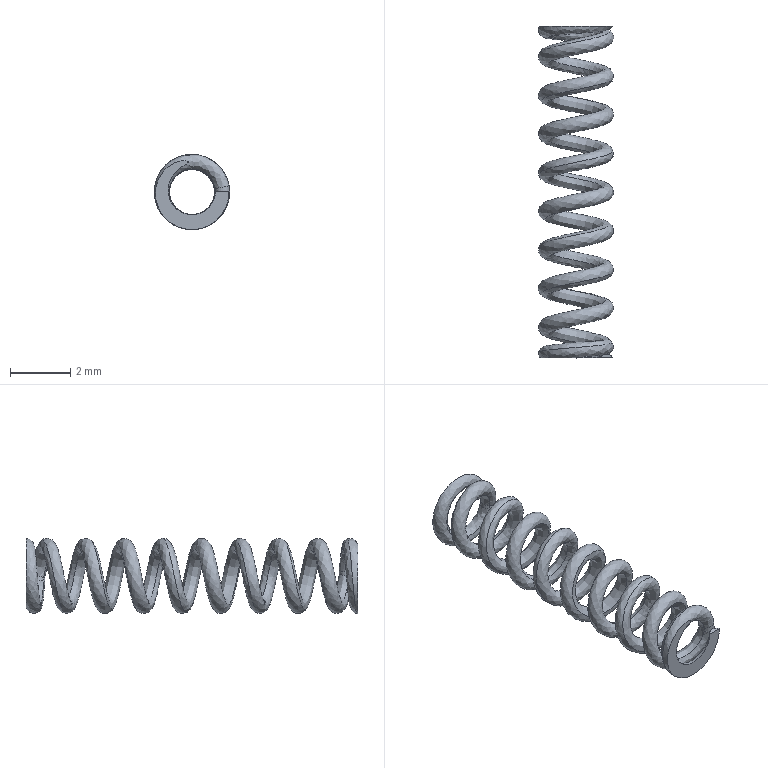Part | SolidWorks | features BaseBody 1 | 1 solid | 14 faces | box 2.498 x 11 x 2.497 mm | volume 11.802 mm3 | spline 10 | plane 4